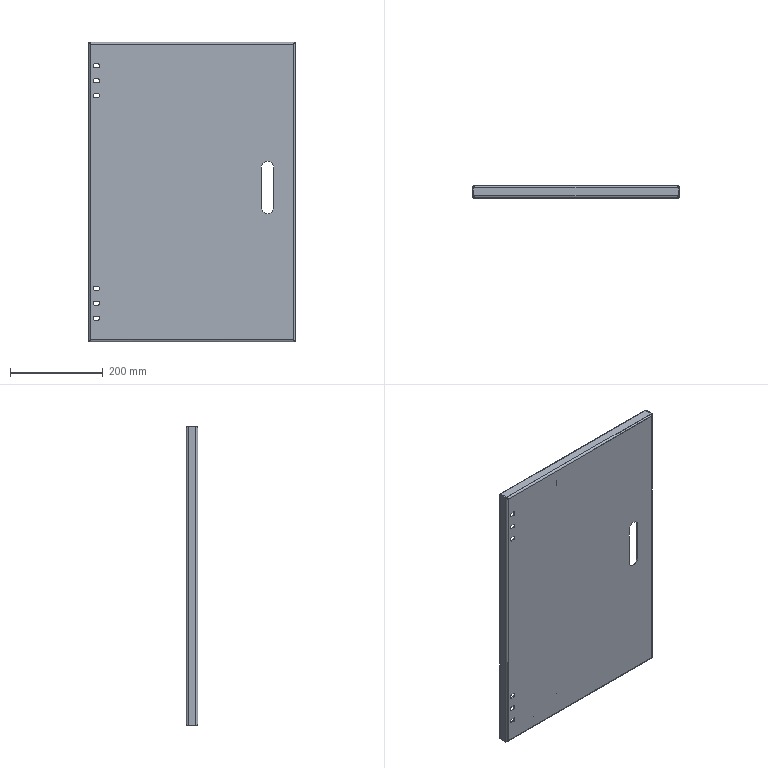Part | SolidWorks | 3 solids | 184 faces | box 445 x 25 x 644 mm | volume 754672 mm3 | plane 104 | cylinder 64 | spline 16 | commonest cylinder face diameters 9 x18 4 x12 7 x12 8 x12 6 x4 10 x4